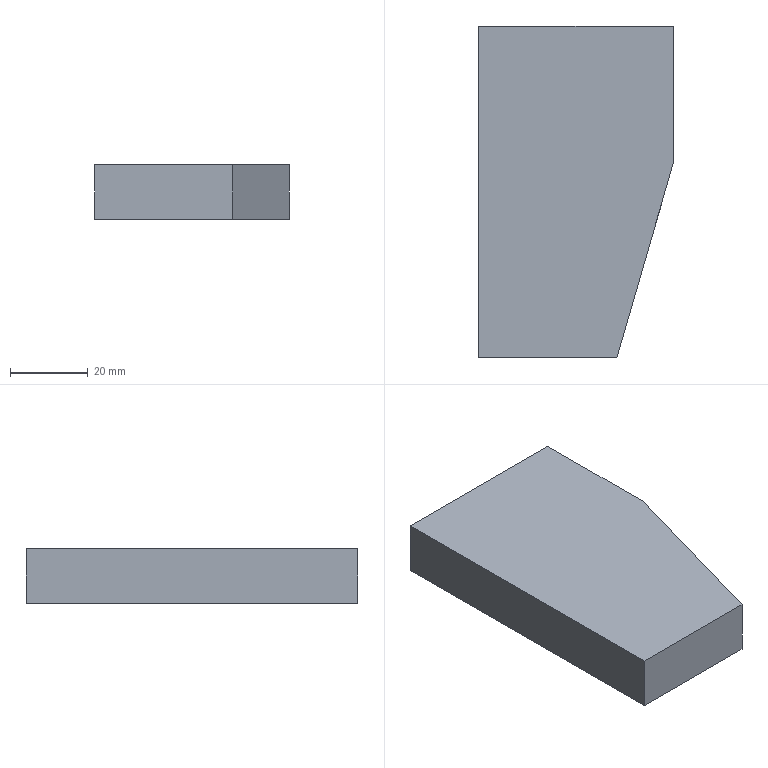Part | SolidWorks | features Extrusion 1 | 1 solid | 7 faces | box 50 x 85 x 14 mm | volume 54425 mm3 | plane 7
STEP:
#1=CARTESIAN_POINT('',(0.,0.,0.));
#2=VERTEX_POINT('',#1);
#3=CARTESIAN_POINT('',(35.5,0.,0.));
#4=VERTEX_POINT('',#3);
#5=CARTESIAN_POINT('',(35.5,0.,0.));
#6=DIRECTION('',(1.,0.,0.));
#7=VECTOR('',#6,1000.);
#8=LINE('',#5,#7);
#9=EDGE_CURVE('',#2,#4,#8,.T.);
#10=ORIENTED_EDGE('',*,*,#9,.T.);
#11=CARTESIAN_POINT('',(35.5,0.,14.));
#12=VERTEX_POINT('',#11);
#13=CARTESIAN_POINT('',(35.5,0.,14.));
#14=DIRECTION('',(0.,0.,-1.));
#15=VECTOR('',#14,1000.);
#16=LINE('',#13,#15);
#17=EDGE_CURVE('',#12,#4,#16,.T.);
#18=ORIENTED_EDGE('',*,*,#17,.F.);
#19=CARTESIAN_POINT('',(0.,0.,14.));
#20=VERTEX_POINT('',#19);
#21=CARTESIAN_POINT('',(35.5,0.,14.));
#22=DIRECTION('',(1.,0.,0.));
#23=VECTOR('',#22,1000.);
#24=LINE('',#21,#23);
#25=EDGE_CURVE('',#20,#12,#24,.T.);
#26=ORIENTED_EDGE('',*,*,#25,.F.);
#27=CARTESIAN_POINT('',(0.,0.,14.));
#28=DIRECTION('',(0.,0.,-1.));
#29=VECTOR('',#28,1000.);
#30=LINE('',#27,#29);
#31=EDGE_CURVE('',#20,#2,#30,.T.);
#32=ORIENTED_EDGE('',*,*,#31,.T.);
#33=EDGE_LOOP('',(#10,#18,#26,#32));
#34=FACE_OUTER_BOUND('',#33,.T.);
#35=CARTESIAN_POINT('',(35.5,0.,14.));
#36=DIRECTION('',(0.,1.,0.));
#37=DIRECTION('',(0.,0.,1.));
#38=AXIS2_PLACEMENT_3D('',#35,#36,#37);
#39=PLANE('',#38);
#40=ADVANCED_FACE('',(#34),#39,.F.);
#41=CARTESIAN_POINT('',(50.,50.,0.));
#42=VERTEX_POINT('',#41);
#43=CARTESIAN_POINT('',(50.,50.,0.));
#44=DIRECTION('',(0.2785,0.9604,0.));
#45=VECTOR('',#44,1000.);
#46=LINE('',#43,#45);
#47=EDGE_CURVE('',#4,#42,#46,.T.);
#48=ORIENTED_EDGE('',*,*,#47,.T.);
#49=CARTESIAN_POINT('',(50.,50.,14.));
#50=VERTEX_POINT('',#49);
#51=CARTESIAN_POINT('',(50.,50.,14.));
#52=DIRECTION('',(0.,0.,-1.));
#53=VECTOR('',#52,1000.);
#54=LINE('',#51,#53);
#55=EDGE_CURVE('',#50,#42,#54,.T.);
#56=ORIENTED_EDGE('',*,*,#55,.F.);
#57=CARTESIAN_POINT('',(50.,50.,14.));
#58=DIRECTION('',(0.2785,0.9604,0.));
#59=VECTOR('',#58,1000.);
#60=LINE('',#57,#59);
#61=EDGE_CURVE('',#12,#50,#60,.T.);
#62=ORIENTED_EDGE('',*,*,#61,.F.);
#63=ORIENTED_EDGE('',*,*,#17,.T.);
#64=EDGE_LOOP('',(#48,#56,#62,#63));
#65=FACE_OUTER_BOUND('',#64,.T.);
#66=CARTESIAN_POINT('',(50.,50.,14.));
#67=DIRECTION('',(-0.9604,0.2785,0.));
#68=DIRECTION('',(-0.2785,-0.9604,0.));
#69=AXIS2_PLACEMENT_3D('',#66,#67,#68);
#70=PLANE('',#69);
#71=ADVANCED_FACE('',(#65),#70,.F.);
#72=CARTESIAN_POINT('',(50.,85.,0.));
#73=VERTEX_POINT('',#72);
#74=CARTESIAN_POINT('',(50.,85.,0.));
#75=DIRECTION('',(0.,1.,0.));
#76=VECTOR('',#75,1000.);
#77=LINE('',#74,#76);
#78=EDGE_CURVE('',#42,#73,#77,.T.);
#79=ORIENTED_EDGE('',*,*,#78,.T.);
#80=CARTESIAN_POINT('',(50.,85.,14.));
#81=VERTEX_POINT('',#80);
#82=CARTESIAN_POINT('',(50.,85.,14.));
#83=DIRECTION('',(0.,0.,-1.));
#84=VECTOR('',#83,1000.);
#85=LINE('',#82,#84);
#86=EDGE_CURVE('',#81,#73,#85,.T.);
#87=ORIENTED_EDGE('',*,*,#86,.F.);
#88=CARTESIAN_POINT('',(50.,85.,14.));
#89=DIRECTION('',(0.,1.,0.));
#90=VECTOR('',#89,1000.);
#91=LINE('',#88,#90);
#92=EDGE_CURVE('',#50,#81,#91,.T.);
#93=ORIENTED_EDGE('',*,*,#92,.F.);
#94=ORIENTED_EDGE('',*,*,#55,.T.);
#95=EDGE_LOOP('',(#79,#87,#93,#94));
#96=FACE_OUTER_BOUND('',#95,.T.);
#97=CARTESIAN_POINT('',(50.,85.,14.));
#98=DIRECTION('',(-1.,0.,0.));
#99=DIRECTION('',(0.,-1.,0.));
#100=AXIS2_PLACEMENT_3D('',#97,#98,#99);
#101=PLANE('',#100);
#102=ADVANCED_FACE('',(#96),#101,.F.);
#103=CARTESIAN_POINT('',(0.,85.,0.));
#104=VERTEX_POINT('',#103);
#105=CARTESIAN_POINT('',(0.,85.,0.));
#106=DIRECTION('',(-1.,0.,0.));
#107=VECTOR('',#106,1000.);
#108=LINE('',#105,#107);
#109=EDGE_CURVE('',#73,#104,#108,.T.);
#110=ORIENTED_EDGE('',*,*,#109,.T.);
#111=CARTESIAN_POINT('',(0.,85.,14.));
#112=VERTEX_POINT('',#111);
#113=CARTESIAN_POINT('',(0.,85.,14.));
#114=DIRECTION('',(0.,0.,-1.));
#115=VECTOR('',#114,1000.);
#116=LINE('',#113,#115);
#117=EDGE_CURVE('',#112,#104,#116,.T.);
#118=ORIENTED_EDGE('',*,*,#117,.F.);
#119=CARTESIAN_POINT('',(0.,85.,14.));
#120=DIRECTION('',(-1.,0.,0.));
#121=VECTOR('',#120,1000.);
#122=LINE('',#119,#121);
#123=EDGE_CURVE('',#81,#112,#122,.T.);
#124=ORIENTED_EDGE('',*,*,#123,.F.);
#125=ORIENTED_EDGE('',*,*,#86,.T.);
#126=EDGE_LOOP('',(#110,#118,#124,#125));
#127=FACE_OUTER_BOUND('',#126,.T.);
#128=CARTESIAN_POINT('',(0.,85.,14.));
#129=DIRECTION('',(0.,-1.,0.));
#130=DIRECTION('',(0.,0.,-1.));
#131=AXIS2_PLACEMENT_3D('',#128,#129,#130);
#132=PLANE('',#131);
#133=ADVANCED_FACE('',(#127),#132,.F.);
#134=CARTESIAN_POINT('',(0.,0.,0.));
#135=DIRECTION('',(0.,-1.,0.));
#136=VECTOR('',#135,1000.);
#137=LINE('',#134,#136);
#138=EDGE_CURVE('',#104,#2,#137,.T.);
#139=ORIENTED_EDGE('',*,*,#138,.T.);
#140=ORIENTED_EDGE('',*,*,#31,.F.);
#141=CARTESIAN_POINT('',(0.,0.,14.));
#142=DIRECTION('',(0.,-1.,0.));
#143=VECTOR('',#142,1000.);
#144=LINE('',#141,#143);
#145=EDGE_CURVE('',#112,#20,#144,.T.);
#146=ORIENTED_EDGE('',*,*,#145,.F.);
#147=ORIENTED_EDGE('',*,*,#117,.T.);
#148=EDGE_LOOP('',(#139,#140,#146,#147));
#149=FACE_OUTER_BOUND('',#148,.T.);
#150=CARTESIAN_POINT('',(0.,0.,14.));
#151=DIRECTION('',(1.,0.,0.));
#152=DIRECTION('',(0.,1.,0.));
#153=AXIS2_PLACEMENT_3D('',#150,#151,#152);
#154=PLANE('',#153);
#155=ADVANCED_FACE('',(#149),#154,.F.);
#156=ORIENTED_EDGE('',*,*,#25,.T.);
#157=ORIENTED_EDGE('',*,*,#61,.T.);
#158=ORIENTED_EDGE('',*,*,#92,.T.);
#159=ORIENTED_EDGE('',*,*,#123,.T.);
#160=ORIENTED_EDGE('',*,*,#145,.T.);
#161=EDGE_LOOP('',(#156,#157,#158,#159,#160));
#162=FACE_OUTER_BOUND('',#161,.T.);
#163=CARTESIAN_POINT('',(0.,0.,14.));
#164=DIRECTION('',(0.,0.,-1.));
#165=DIRECTION('',(-1.,0.,0.));
#166=AXIS2_PLACEMENT_3D('',#163,#164,#165);
#167=PLANE('',#166);
#168=ADVANCED_FACE('',(#162),#167,.F.);
#169=ORIENTED_EDGE('',*,*,#9,.F.);
#170=ORIENTED_EDGE('',*,*,#138,.F.);
#171=ORIENTED_EDGE('',*,*,#109,.F.);
#172=ORIENTED_EDGE('',*,*,#78,.F.);
#173=ORIENTED_EDGE('',*,*,#47,.F.);
#174=EDGE_LOOP('',(#169,#170,#171,#172,#173));
#175=FACE_OUTER_BOUND('',#174,.T.);
#176=CARTESIAN_POINT('',(0.,0.,0.));
#177=DIRECTION('',(0.,0.,-1.));
#178=DIRECTION('',(-1.,0.,0.));
#179=AXIS2_PLACEMENT_3D('',#176,#177,#178);
#180=PLANE('',#179);
#181=ADVANCED_FACE('',(#175),#180,.T.);
#182=CLOSED_SHELL('',(#40,#71,#102,#133,#155,#168,#181));
#183=MANIFOLD_SOLID_BREP('',#182);
#184=CARTESIAN_POINT('',(0.,0.,0.));
#185=DIRECTION('',(0.,0.,1.));
#186=DIRECTION('',(1.,0.,0.));
#187=AXIS2_PLACEMENT_3D('',#184,#185,#186);
#188=(LENGTH_UNIT()NAMED_UNIT(*)SI_UNIT(.MILLI.,.METRE.));
#189=UNCERTAINTY_MEASURE_WITH_UNIT(LENGTH_MEASURE(0.00001),#188,'','');
#190=(NAMED_UNIT(*)PLANE_ANGLE_UNIT()SI_UNIT($,.RADIAN.));
#191=(NAMED_UNIT(*)SI_UNIT($,.STERADIAN.)SOLID_ANGLE_UNIT());
#192=(GEOMETRIC_REPRESENTATION_CONTEXT(3)GLOBAL_UNCERTAINTY_ASSIGNED_CONTEXT((#189))GLOBAL_UNIT_ASSIGNED_CONTEXT((#188,#190,#191))REPRESENTATION_CONTEXT('',''));
#193=ADVANCED_BREP_SHAPE_REPRESENTATION('',(#183,#187),#192);